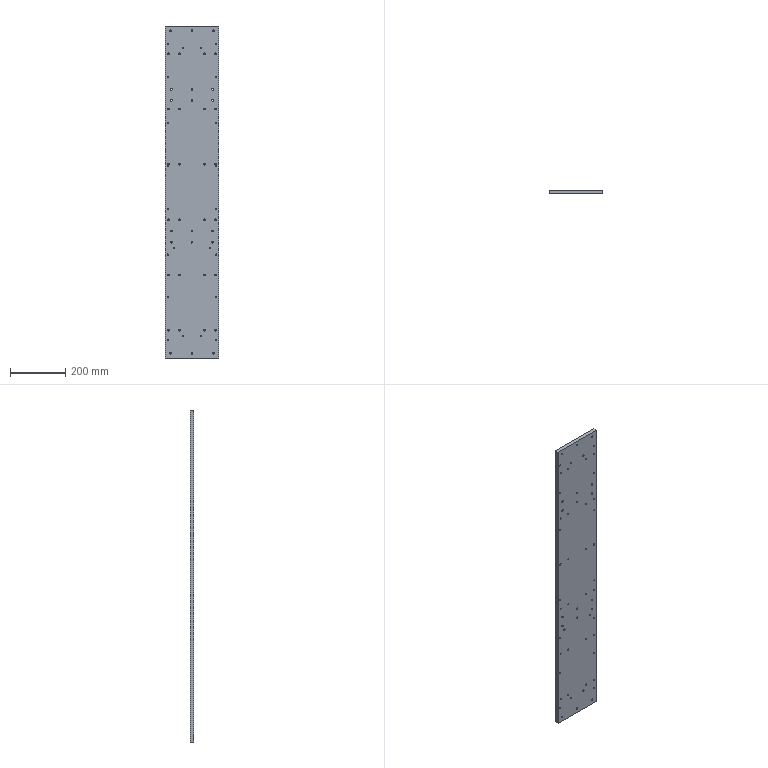Part | SolidWorks | features HoleWzd 6, Extrusion 1, ICE 1 | 1 solid | 134 faces | box 195 x 12 x 1200 mm | volume 2789805 mm3 | cylinder 128 | plane 6 | commonest cylinder face diameters 5 x48 6.8 x36 4.2 x32 6 x12